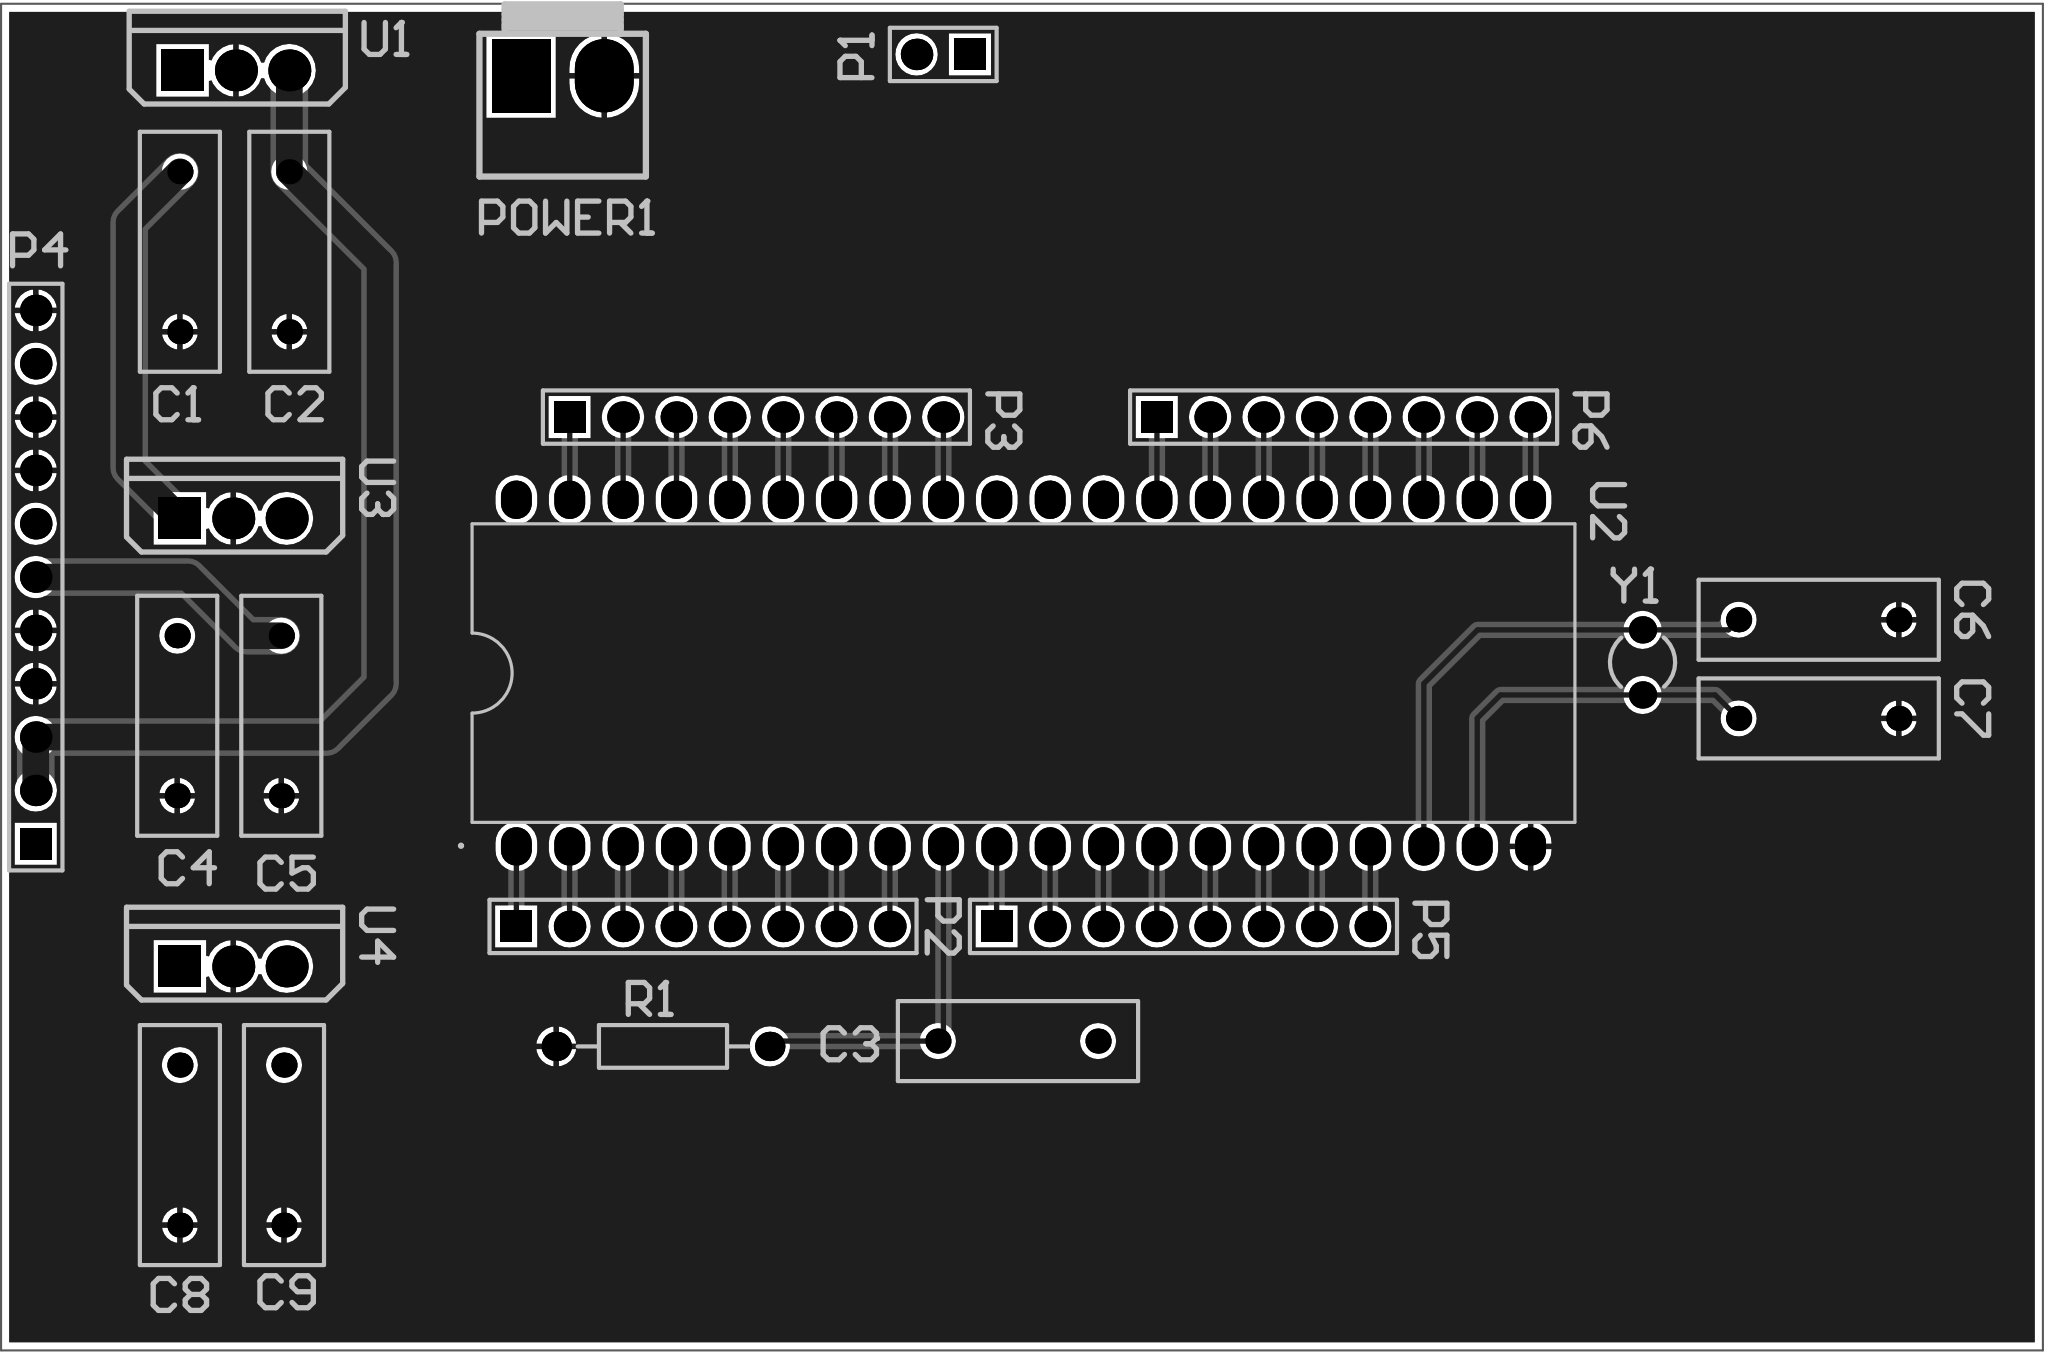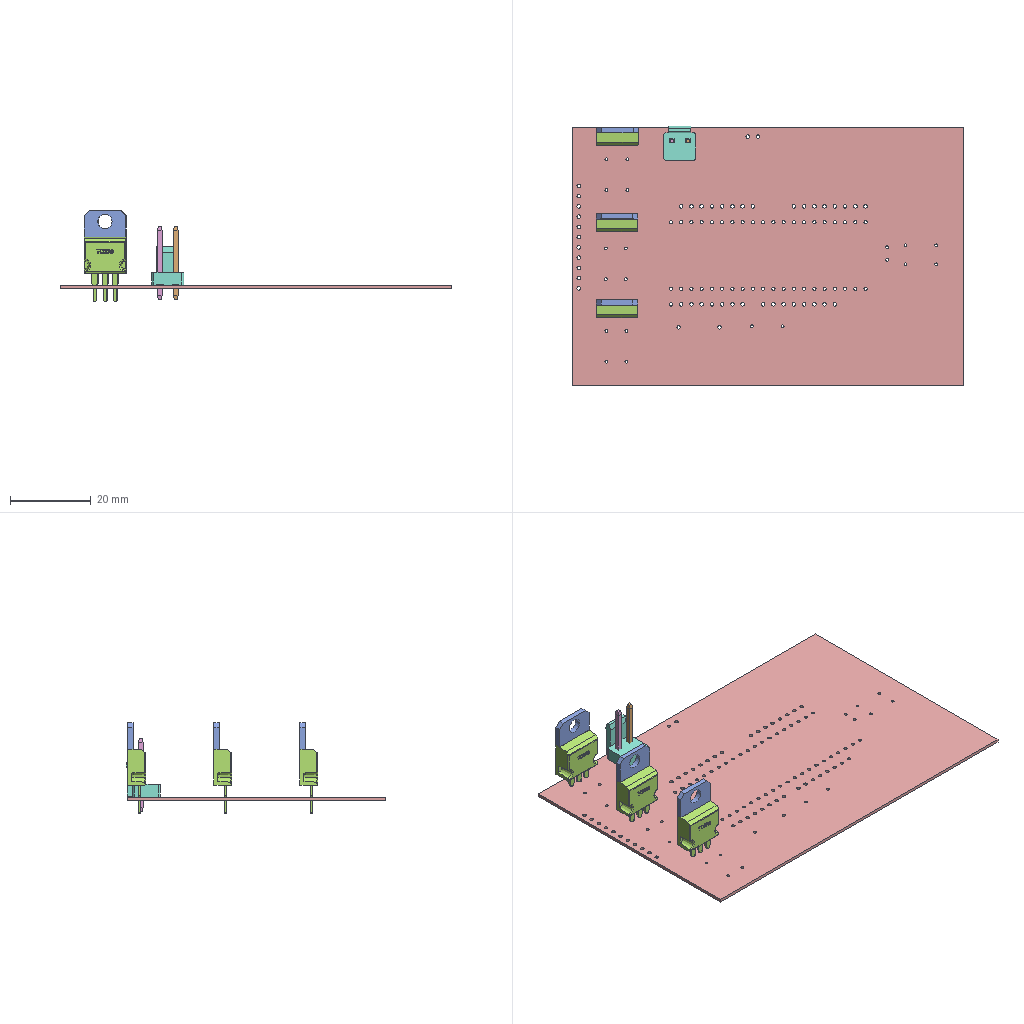Circuit board layout | Altium Designer | box 97.2 x 64.3 x 22.5 mm
Layer stack:
# Altium Designer layer stack of  (unit mm; dielectric type: 0 none, 1 core, 2 prepreg, 3 surface material)
index,name,kind,layer,copper_thickness_mm,dielectric_type,dielectric_thickness_mm,dielectric_material,dielectric_constant
0,Top Paste,other,,,,,,
1,Top Overlay,other,,,,,,
2,Top Solder,dielectric,,,3,0.0102,Solder Resist,3.5
3,Top Layer,copper,Top Layer,0.0356,,,,
4,Dielectric 1,dielectric,,,1,0.254,FR-4,4.2
5,VCC,copper,VCC,0.036,,,,
6,Dielectric 3,dielectric,,,2,0.127,,4.2
7,GND,copper,GND,0.036,,,,
8,Dielectric 2,dielectric,,,1,0.254,,4.2
9,Bottom Layer,copper,Bottom Layer,0.0356,,,,
10,Bottom Solder,dielectric,,,3,0.0102,Solder Resist,3.5
11,Bottom Overlay,other,,,,,,
12,Bottom Paste,other,,,,,,
# drill layer pairs: low layer,high layer
drill_pair,Top Layer,Bottom Layer
Part placement:
Designator,Comment,Layer,Footprint,Center-X(mm),Center-Y(mm),Rotation
Y1,XTAL,TopLayer,R38,125.095,64.516,180
U4,LM7806,TopLayer,TO220A,58.039,50.038,360
U3,LM7805,TopLayer,TO220A,58.039,71.374,360
U2,STC89C52RC,TopLayer,STC89C52RC,95.639,64.008,360
U1,LM7805,TopLayer,TO220A,58.166,92.71,360
R1,10K,TopLayer,AXIAL-0.4,78.486,46.228,360
POWER1,Terminal block,TopLayer,VH3.96-2A,73.712,92.456,360
P6,Header 8,TopLayer,HDR1X8,110.871,76.2,360
P5,Header 8,TopLayer,HDR1X8,103.251,51.943,360
P4,Header 11,TopLayer,HDR1X11,48.641,68.58,90
P3,Header 8,TopLayer,HDR1X8,82.931,76.2,360
P2,Header 8,TopLayer,HDR1X8,80.391,51.943,360
P1,Header 2,TopLayer,HDR1X2,91.821,93.472,180
C9,0.1UF,TopLayer,RAD-0.3,60.452,41.529,270
C8,0.33UF,TopLayer,RAD-0.3,55.499,41.529,270
C7,22pF,TopLayer,RAD-0.3,133.477,61.849,360
C6,22pF,TopLayer,RAD-0.3,133.477,66.548,360
C5,0.1UF,TopLayer,RAD-0.3,60.325,61.976,270
C4,0.33UF,TopLayer,RAD-0.3,55.372,61.976,270
C3,10UF,TopLayer,RAD-0.3,95.377,46.482,180
C2,0.1UF,TopLayer,RAD-0.3,60.706,84.074,270
C1,0.33UF,TopLayer,RAD-0.3,55.499,84.074,270
Pad and via stacks:
# Altium Designer via and pad stacks of  (unit mm). Each distinct definition once, with the count of objects using it.
# via: kind,start_layer,end_layer,hole_mm,diameter_mm,mode(0 simple;1 top-mid-bottom;2 full stack),diameter_per_layer,count,example_net
# pad: kind,layer,hole_mm,hole_type(0 round;1 square;2 slot),plating,top_size,top_shape(1 round;2 rect;3 octagon;9 rounded rect),mid_size,bottom_size,mode,footprint,size_per_layer,count,example
pad,Multi-Layer,0.9,0,plated,1.5x1.5,2,1.5x1.5,1.5x1.5,0,HDR1X8,,4,P3.1
pad,Multi-Layer,0.9,0,plated,1.5x1.5,1,1.5x1.5,1.5x1.5,0,HDR1X8,,28,P3.2
pad,Multi-Layer,0.7,0,plated,1.2x1.2,1,1.2x1.2,1.2x1.2,0,RAD-0.3,,18,C2.2
pad,Multi-Layer,1.1,0,plated,2x2,1,2x2,2x2,0,TO220A,,6,U3.2
pad,Multi-Layer,1.1,0,plated,2x2,2,2x2,2x2,0,TO220A,,3,U3.1
pad,Multi-Layer,0.9,0,plated,1.5x1.5,2,1.5x1.5,1.5x1.5,0,HDR1X2,,1,P1.1
pad,Multi-Layer,0.9,0,plated,1.5x1.5,1,1.5x1.5,1.5x1.5,0,HDR1X2,,1,P1.2
pad,Multi-Layer,0.9,0,plated,1.5x1.5,1,1.5x1.5,1.5x1.5,0,HDR1X11,,10,P4.11
pad,Multi-Layer,0.9,0,plated,1.5x1.5,2,1.5x1.5,1.5x1.5,0,HDR1X11,,1,P4.1
pad,Multi-Layer,1.6,0,plated,2.8x3.5,2,2.8x3.5,2.8x3.5,0,VH3.96-2A,,1,POWER1.1
pad,Multi-Layer,1.6,0,plated,2.8x3.5,1,2.8x3.5,2.8x3.5,0,VH3.96-2A,,1,POWER1.2
pad,Multi-Layer,0.85,0,plated,1.4x1.4,1,1.4x1.4,1.4x1.4,0,AXIAL-0.4,,2,R1.1
pad,Multi-Layer,0.8,0,plated,1.467x1.833,1,1.467x1.833,1.467x1.833,0,STC89C52RC,,40,U2.1
pad,Multi-Layer,0.7,0,plated,1.3x1.3,1,1.3x1.3,1.3x1.3,0,R38,,2,Y1.1
Copper pours:
name,layer,net,type(0 solid;1 hatched;2 none)
D,Top Layer,GND,0
D,Bottom Layer,GND,0
Design rules, without the lines most boards share:
# Altium Designer design rules of  (exported by Altium Designer, unit mm)
# columns: name | kind | enabled | priority | scope1 | scope2 | descriptor | typed fields (field=value)
SilkToSilkClearance | 55 | enabled | 1 | All | All | Silk to Silk (Clearance=0mil) (All),(All) |
SilkToSolderMaskClearance | 54 | enabled | 1 | IsPad | All | Silk To Solder Mask (Clearance=0mil) (IsPad),(All) |
MinimumSolderMaskSliver | 53 | enabled | 1 | All | All | Minimum Solder Mask Sliver (Gap=0mil) (All),(All) |
HoleToHoleClearance | 52 | enabled | 1 | All | All | Hole To Hole Clearance (Gap=10mil) (All),(All) | gap=0.254
DiffPairsRouting | 51 | enabled | 1 | All | All | Differential Pairs Uncoupled Length using the Gap Constraints (Min=10mil) (Max=10mil) (Prefered=10mil)  and Width Constraints (Min=15mil) (Max=15mil) (Prefered=15mil) (All) |
SolderMaskExpansion | 13 | enabled | 1 | All | All | Solder Mask Expansion (Expansion =4mil) (All) | expansion=0.1016
RoutingVias | 11 | enabled | 1 | All | All | Routing Via (MinHoleWidth=28mil) (MaxHoleWidth=28mil) (PreferredHoleWidth=28mil) (MinWidth=50mil) (MaxWidth=50mil) (PreferedWidth=50mil) (All) | via_min_hole=0.7112 via_max_hole=0.7112 via_preferred_diameter=1.27 via_preferred_hole=0.7112
Width | 2 | enabled | 1 | All | All | Width Constraint (Min=10mil) (Max=50mil) (Preferred=10mil) (All) |
PolygonConnect | 20 | enabled | 1 | All | All | Polygon Connect Rule(Relief Connect )(Conductor Width=10mil) (Relief Angle=90 Angle) (Entries=4) (Air Gap Width=10mil) (All),(All) | connect_style(0=relief,1=direct,2=none)=0 relief_conductor_width=0.254 relief_entries=4
PlaneConnect | 6 | enabled | 1 | All | All | Power Plane Connect Rule(Relief Connect )(Expansion=20mil) (Conductor Width=10mil) (Air Gap=10mil) (Entries=4) (All) | relief_conductor_width=0.254 relief_entries=4 relief_expansion=0.508
Clearance | 0 | enabled | 1 | All | All | Clearance Constraint (Gap=10mil) (All),(All) | gap=0.254
Classes set for this board:
# Altium Designer classes of  (member kind: 0 net, 1 component, 2 from-to, 3 pad, 4 layer, 5 differential pair, 6 design channel, 7 polygon, 8 structure, 9 xSignal)
# columns: class name | member kind | superclass | members
Sheet1 | 1 | no | C1; C2; C3; C4; C5; C6; C7; C8; C9; P1; P2; P3; P4; P5; P6; POWER1; R1; U1; U2; U3; U4; Y1;